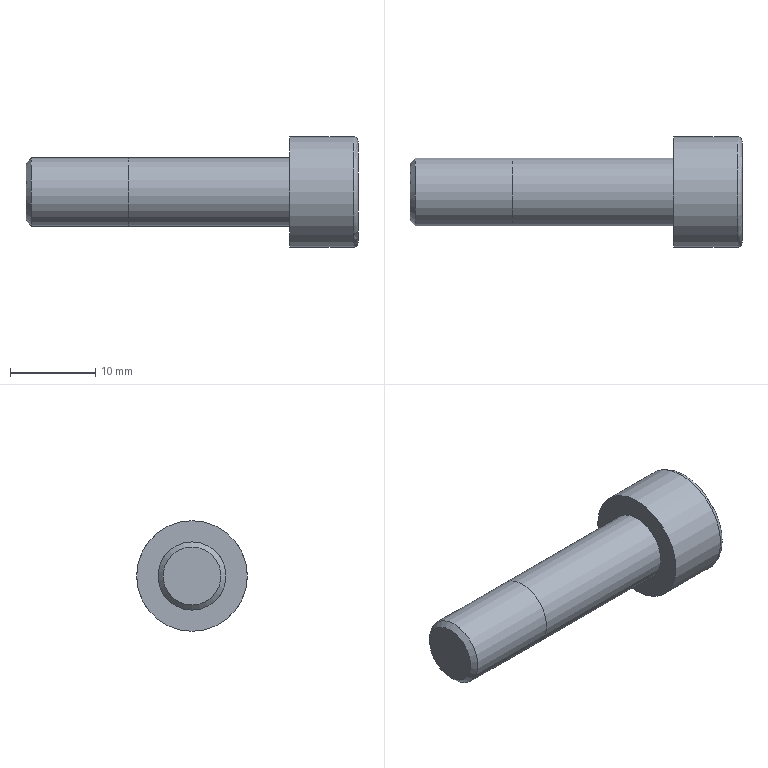Part | STEP file | solid 3 | 1 solid | 21 faces | box 39 x 13 x 13 mm | volume 2314 mm3 | plane 14 | cylinder 5 | torus 1 | cone 1 | commonest cylinder face diameters 6.8 x1 6.98 x1 7.99 x1 8 x1 13 x1